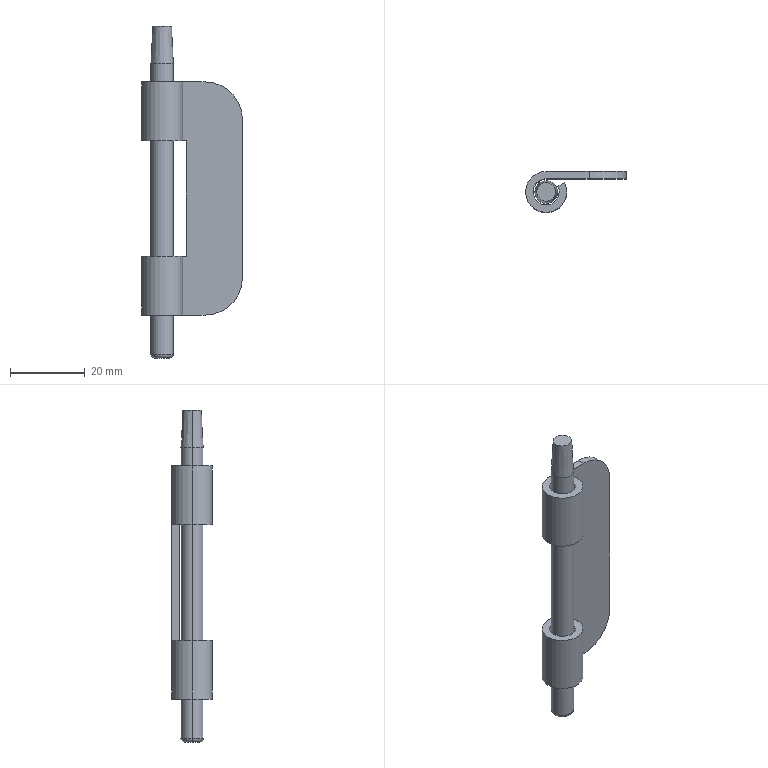Part | SolidWorks | features ICE 3, Chamfer 2, Fillet 2, ExtruThin 1 | 2 solids | 32 faces | box 27 x 11 x 89 mm | volume 6132 mm3 | cylinder 16 | plane 12 | torus 2 | cone 2 | commonest cylinder face diameters 7 x6 11 x6 6 x2 20 x2
STEP:
#1=CARTESIAN_POINT('',(-3.5,-3.5,31.25));
#2=VERTEX_POINT('',#1);
#3=CARTESIAN_POINT('',(3.5,-3.5,31.25));
#4=VERTEX_POINT('',#3);
#5=CARTESIAN_POINT('',(0.,-3.5,31.25));
#6=DIRECTION('',(0.,0.,1.));
#7=DIRECTION('',(1.,0.,0.));
#8=AXIS2_PLACEMENT_3D('',#5,#6,#7);
#9=CIRCLE('',#8,3.5);
#10=EDGE_CURVE('',#2,#4,#9,.T.);
#11=ORIENTED_EDGE('',*,*,#10,.T.);
#12=CARTESIAN_POINT('',(3.5,-3.5,15.5));
#13=VERTEX_POINT('',#12);
#14=CARTESIAN_POINT('',(3.5,-3.5,31.25));
#15=DIRECTION('',(0.,0.,-1.));
#16=VECTOR('',#15,1000.);
#17=LINE('',#14,#16);
#18=EDGE_CURVE('',#4,#13,#17,.T.);
#19=ORIENTED_EDGE('',*,*,#18,.T.);
#20=CARTESIAN_POINT('',(-3.5,-3.5,15.5));
#21=VERTEX_POINT('',#20);
#22=CARTESIAN_POINT('',(0.,-3.5,15.5));
#23=DIRECTION('',(0.,0.,1.));
#24=DIRECTION('',(1.,0.,0.));
#25=AXIS2_PLACEMENT_3D('',#22,#23,#24);
#26=CIRCLE('',#25,3.5);
#27=EDGE_CURVE('',#21,#13,#26,.T.);
#28=ORIENTED_EDGE('',*,*,#27,.F.);
#29=CARTESIAN_POINT('',(-3.5,-3.5,31.25));
#30=DIRECTION('',(0.,0.,-1.));
#31=VECTOR('',#30,1000.);
#32=LINE('',#29,#31);
#33=EDGE_CURVE('',#2,#21,#32,.T.);
#34=ORIENTED_EDGE('',*,*,#33,.F.);
#35=EDGE_LOOP('',(#11,#19,#28,#34));
#36=FACE_OUTER_BOUND('',#35,.T.);
#37=CARTESIAN_POINT('',(0.,-3.5,31.25));
#38=DIRECTION('',(0.,0.,-1.));
#39=DIRECTION('',(-1.,0.,0.));
#40=AXIS2_PLACEMENT_3D('',#37,#38,#39);
#41=CYLINDRICAL_SURFACE('',#40,3.5);
#42=ADVANCED_FACE('',(#36),#41,.F.);
#43=CARTESIAN_POINT('',(0.,0.,31.25));
#44=VERTEX_POINT('',#43);
#45=CARTESIAN_POINT('',(0.,-3.5,31.25));
#46=DIRECTION('',(0.,0.,1.));
#47=DIRECTION('',(1.,0.,0.));
#48=AXIS2_PLACEMENT_3D('',#45,#46,#47);
#49=CIRCLE('',#48,3.5);
#50=EDGE_CURVE('',#44,#2,#49,.T.);
#51=ORIENTED_EDGE('',*,*,#50,.T.);
#52=ORIENTED_EDGE('',*,*,#33,.T.);
#53=CARTESIAN_POINT('',(0.,0.,15.5));
#54=VERTEX_POINT('',#53);
#55=CARTESIAN_POINT('',(0.,-3.5,15.5));
#56=DIRECTION('',(0.,0.,1.));
#57=DIRECTION('',(1.,0.,0.));
#58=AXIS2_PLACEMENT_3D('',#55,#56,#57);
#59=CIRCLE('',#58,3.5);
#60=EDGE_CURVE('',#54,#21,#59,.T.);
#61=ORIENTED_EDGE('',*,*,#60,.F.);
#62=CARTESIAN_POINT('',(0.,0.,31.25));
#63=DIRECTION('',(0.,0.,-1.));
#64=VECTOR('',#63,1000.);
#65=LINE('',#62,#64);
#66=EDGE_CURVE('',#44,#54,#65,.T.);
#67=ORIENTED_EDGE('',*,*,#66,.F.);
#68=EDGE_LOOP('',(#51,#52,#61,#67));
#69=FACE_OUTER_BOUND('',#68,.T.);
#70=CARTESIAN_POINT('',(0.,-3.5,31.25));
#71=DIRECTION('',(0.,0.,-1.));
#72=DIRECTION('',(-1.,0.,0.));
#73=AXIS2_PLACEMENT_3D('',#70,#71,#72);
#74=CYLINDRICAL_SURFACE('',#73,3.5);
#75=ADVANCED_FACE('',(#69),#74,.F.);
#76=CARTESIAN_POINT('',(4.939,-1.08,-15.5));
#77=VERTEX_POINT('',#76);
#78=CARTESIAN_POINT('',(5.5,-3.5,-15.5));
#79=VERTEX_POINT('',#78);
#80=CARTESIAN_POINT('',(0.,-3.5,-15.5));
#81=DIRECTION('',(0.,0.,-1.));
#82=DIRECTION('',(-1.,0.,0.));
#83=AXIS2_PLACEMENT_3D('',#80,#81,#82);
#84=CIRCLE('',#83,5.5);
#85=EDGE_CURVE('',#77,#79,#84,.T.);
#86=ORIENTED_EDGE('',*,*,#85,.T.);
#87=CARTESIAN_POINT('',(5.5,-3.5,-31.25));
#88=VERTEX_POINT('',#87);
#89=CARTESIAN_POINT('',(5.5,-3.5,31.25));
#90=DIRECTION('',(0.,0.,-1.));
#91=VECTOR('',#90,1000.);
#92=LINE('',#89,#91);
#93=EDGE_CURVE('',#79,#88,#92,.T.);
#94=ORIENTED_EDGE('',*,*,#93,.T.);
#95=CARTESIAN_POINT('',(4.939,-1.08,-31.25));
#96=VERTEX_POINT('',#95);
#97=CARTESIAN_POINT('',(0.,-3.5,-31.25));
#98=DIRECTION('',(0.,0.,1.));
#99=DIRECTION('',(1.,0.,0.));
#100=AXIS2_PLACEMENT_3D('',#97,#98,#99);
#101=CIRCLE('',#100,5.5);
#102=EDGE_CURVE('',#88,#96,#101,.T.);
#103=ORIENTED_EDGE('',*,*,#102,.T.);
#104=CARTESIAN_POINT('',(4.939,-1.08,31.25));
#105=DIRECTION('',(0.,0.,-1.));
#106=VECTOR('',#105,1000.);
#107=LINE('',#104,#106);
#108=EDGE_CURVE('',#77,#96,#107,.T.);
#109=ORIENTED_EDGE('',*,*,#108,.F.);
#110=EDGE_LOOP('',(#86,#94,#103,#109));
#111=FACE_OUTER_BOUND('',#110,.T.);
#112=CARTESIAN_POINT('',(0.,-3.5,31.25));
#113=DIRECTION('',(0.,0.,-1.));
#114=DIRECTION('',(-1.,0.,0.));
#115=AXIS2_PLACEMENT_3D('',#112,#113,#114);
#116=CYLINDRICAL_SURFACE('',#115,5.5);
#117=ADVANCED_FACE('',(#111),#116,.T.);
#118=ORIENTED_EDGE('',*,*,#93,.F.);
#119=CARTESIAN_POINT('',(-5.5,-3.5,-15.5));
#120=VERTEX_POINT('',#119);
#121=CARTESIAN_POINT('',(0.,-3.5,-15.5));
#122=DIRECTION('',(0.,0.,-1.));
#123=DIRECTION('',(-1.,0.,0.));
#124=AXIS2_PLACEMENT_3D('',#121,#122,#123);
#125=CIRCLE('',#124,5.5);
#126=EDGE_CURVE('',#79,#120,#125,.T.);
#127=ORIENTED_EDGE('',*,*,#126,.T.);
#128=CARTESIAN_POINT('',(-5.5,-3.5,-31.25));
#129=VERTEX_POINT('',#128);
#130=CARTESIAN_POINT('',(-5.5,-3.5,31.25));
#131=DIRECTION('',(0.,0.,-1.));
#132=VECTOR('',#131,1000.);
#133=LINE('',#130,#132);
#134=EDGE_CURVE('',#120,#129,#133,.T.);
#135=ORIENTED_EDGE('',*,*,#134,.T.);
#136=CARTESIAN_POINT('',(0.,-3.5,-31.25));
#137=DIRECTION('',(0.,0.,1.));
#138=DIRECTION('',(1.,0.,0.));
#139=AXIS2_PLACEMENT_3D('',#136,#137,#138);
#140=CIRCLE('',#139,5.5);
#141=EDGE_CURVE('',#129,#88,#140,.T.);
#142=ORIENTED_EDGE('',*,*,#141,.T.);
#143=EDGE_LOOP('',(#118,#127,#135,#142));
#144=FACE_OUTER_BOUND('',#143,.T.);
#145=CARTESIAN_POINT('',(0.,-3.5,31.25));
#146=DIRECTION('',(0.,0.,-1.));
#147=DIRECTION('',(-1.,0.,0.));
#148=AXIS2_PLACEMENT_3D('',#145,#146,#147);
#149=CYLINDRICAL_SURFACE('',#148,5.5);
#150=ADVANCED_FACE('',(#144),#149,.T.);
#151=CARTESIAN_POINT('',(3.5,-3.5,-15.5));
#152=VERTEX_POINT('',#151);
#153=CARTESIAN_POINT('',(-3.5,-3.5,-15.5));
#154=VERTEX_POINT('',#153);
#155=CARTESIAN_POINT('',(0.,-3.5,-15.5));
#156=DIRECTION('',(0.,0.,-1.));
#157=DIRECTION('',(-1.,0.,0.));
#158=AXIS2_PLACEMENT_3D('',#155,#156,#157);
#159=CIRCLE('',#158,3.5);
#160=EDGE_CURVE('',#152,#154,#159,.T.);
#161=ORIENTED_EDGE('',*,*,#160,.F.);
#162=CARTESIAN_POINT('',(3.5,-3.5,-31.25));
#163=VERTEX_POINT('',#162);
#164=CARTESIAN_POINT('',(3.5,-3.5,31.25));
#165=DIRECTION('',(0.,0.,-1.));
#166=VECTOR('',#165,1000.);
#167=LINE('',#164,#166);
#168=EDGE_CURVE('',#152,#163,#167,.T.);
#169=ORIENTED_EDGE('',*,*,#168,.T.);
#170=CARTESIAN_POINT('',(-3.5,-3.5,-31.25));
#171=VERTEX_POINT('',#170);
#172=CARTESIAN_POINT('',(0.,-3.5,-31.25));
#173=DIRECTION('',(0.,0.,1.));
#174=DIRECTION('',(1.,0.,0.));
#175=AXIS2_PLACEMENT_3D('',#172,#173,#174);
#176=CIRCLE('',#175,3.5);
#177=EDGE_CURVE('',#171,#163,#176,.T.);
#178=ORIENTED_EDGE('',*,*,#177,.F.);
#179=CARTESIAN_POINT('',(-3.5,-3.5,31.25));
#180=DIRECTION('',(0.,0.,-1.));
#181=VECTOR('',#180,1000.);
#182=LINE('',#179,#181);
#183=EDGE_CURVE('',#154,#171,#182,.T.);
#184=ORIENTED_EDGE('',*,*,#183,.F.);
#185=EDGE_LOOP('',(#161,#169,#178,#184));
#186=FACE_OUTER_BOUND('',#185,.T.);
#187=CARTESIAN_POINT('',(0.,-3.5,31.25));
#188=DIRECTION('',(0.,0.,-1.));
#189=DIRECTION('',(-1.,0.,0.));
#190=AXIS2_PLACEMENT_3D('',#187,#188,#189);
#191=CYLINDRICAL_SURFACE('',#190,3.5);
#192=ADVANCED_FACE('',(#186),#191,.F.);
#193=CARTESIAN_POINT('',(0.,0.,-15.5));
#194=VERTEX_POINT('',#193);
#195=CARTESIAN_POINT('',(0.,-3.5,-15.5));
#196=DIRECTION('',(0.,0.,-1.));
#197=DIRECTION('',(-1.,0.,0.));
#198=AXIS2_PLACEMENT_3D('',#195,#196,#197);
#199=CIRCLE('',#198,3.5);
#200=EDGE_CURVE('',#154,#194,#199,.T.);
#201=ORIENTED_EDGE('',*,*,#200,.F.);
#202=ORIENTED_EDGE('',*,*,#183,.T.);
#203=CARTESIAN_POINT('',(0.,0.,-31.25));
#204=VERTEX_POINT('',#203);
#205=CARTESIAN_POINT('',(0.,-3.5,-31.25));
#206=DIRECTION('',(0.,0.,1.));
#207=DIRECTION('',(1.,0.,0.));
#208=AXIS2_PLACEMENT_3D('',#205,#206,#207);
#209=CIRCLE('',#208,3.5);
#210=EDGE_CURVE('',#204,#171,#209,.T.);
#211=ORIENTED_EDGE('',*,*,#210,.F.);
#212=CARTESIAN_POINT('',(0.,0.,31.25));
#213=DIRECTION('',(0.,0.,-1.));
#214=VECTOR('',#213,1000.);
#215=LINE('',#212,#214);
#216=EDGE_CURVE('',#194,#204,#215,.T.);
#217=ORIENTED_EDGE('',*,*,#216,.F.);
#218=EDGE_LOOP('',(#201,#202,#211,#217));
#219=FACE_OUTER_BOUND('',#218,.T.);
#220=CARTESIAN_POINT('',(0.,-3.5,31.25));
#221=DIRECTION('',(0.,0.,-1.));
#222=DIRECTION('',(-1.,0.,0.));
#223=AXIS2_PLACEMENT_3D('',#220,#221,#222);
#224=CYLINDRICAL_SURFACE('',#223,3.5);
#225=ADVANCED_FACE('',(#219),#224,.F.);
#226=CARTESIAN_POINT('',(5.5,-3.5,31.25));
#227=VERTEX_POINT('',#226);
#228=CARTESIAN_POINT('',(4.939,-1.08,31.25));
#229=VERTEX_POINT('',#228);
#230=CARTESIAN_POINT('',(0.,-3.5,31.25));
#231=DIRECTION('',(0.,0.,1.));
#232=DIRECTION('',(1.,0.,0.));
#233=AXIS2_PLACEMENT_3D('',#230,#231,#232);
#234=CIRCLE('',#233,5.5);
#235=EDGE_CURVE('',#227,#229,#234,.T.);
#236=ORIENTED_EDGE('',*,*,#235,.F.);
#237=CARTESIAN_POINT('',(5.5,-3.5,15.5));
#238=VERTEX_POINT('',#237);
#239=CARTESIAN_POINT('',(5.5,-3.5,31.25));
#240=DIRECTION('',(0.,0.,-1.));
#241=VECTOR('',#240,1000.);
#242=LINE('',#239,#241);
#243=EDGE_CURVE('',#227,#238,#242,.T.);
#244=ORIENTED_EDGE('',*,*,#243,.T.);
#245=CARTESIAN_POINT('',(4.939,-1.08,15.5));
#246=VERTEX_POINT('',#245);
#247=CARTESIAN_POINT('',(0.,-3.5,15.5));
#248=DIRECTION('',(0.,0.,1.));
#249=DIRECTION('',(1.,0.,0.));
#250=AXIS2_PLACEMENT_3D('',#247,#248,#249);
#251=CIRCLE('',#250,5.5);
#252=EDGE_CURVE('',#238,#246,#251,.T.);
#253=ORIENTED_EDGE('',*,*,#252,.T.);
#254=CARTESIAN_POINT('',(4.939,-1.08,31.25));
#255=DIRECTION('',(0.,0.,-1.));
#256=VECTOR('',#255,1000.);
#257=LINE('',#254,#256);
#258=EDGE_CURVE('',#229,#246,#257,.T.);
#259=ORIENTED_EDGE('',*,*,#258,.F.);
#260=EDGE_LOOP('',(#236,#244,#253,#259));
#261=FACE_OUTER_BOUND('',#260,.T.);
#262=CARTESIAN_POINT('',(0.,-3.5,31.25));
#263=DIRECTION('',(0.,0.,-1.));
#264=DIRECTION('',(-1.,0.,0.));
#265=AXIS2_PLACEMENT_3D('',#262,#263,#264);
#266=CYLINDRICAL_SURFACE('',#265,5.5);
#267=ADVANCED_FACE('',(#261),#266,.T.);
#268=ORIENTED_EDGE('',*,*,#243,.F.);
#269=CARTESIAN_POINT('',(-5.5,-3.5,31.25));
#270=VERTEX_POINT('',#269);
#271=CARTESIAN_POINT('',(0.,-3.5,31.25));
#272=DIRECTION('',(0.,0.,1.));
#273=DIRECTION('',(1.,0.,0.));
#274=AXIS2_PLACEMENT_3D('',#271,#272,#273);
#275=CIRCLE('',#274,5.5);
#276=EDGE_CURVE('',#270,#227,#275,.T.);
#277=ORIENTED_EDGE('',*,*,#276,.F.);
#278=CARTESIAN_POINT('',(-5.5,-3.5,15.5));
#279=VERTEX_POINT('',#278);
#280=CARTESIAN_POINT('',(-5.5,-3.5,31.25));
#281=DIRECTION('',(0.,0.,-1.));
#282=VECTOR('',#281,1000.);
#283=LINE('',#280,#282);
#284=EDGE_CURVE('',#270,#279,#283,.T.);
#285=ORIENTED_EDGE('',*,*,#284,.T.);
#286=CARTESIAN_POINT('',(0.,-3.5,15.5));
#287=DIRECTION('',(0.,0.,1.));
#288=DIRECTION('',(1.,0.,0.));
#289=AXIS2_PLACEMENT_3D('',#286,#287,#288);
#290=CIRCLE('',#289,5.5);
#291=EDGE_CURVE('',#279,#238,#290,.T.);
#292=ORIENTED_EDGE('',*,*,#291,.T.);
#293=EDGE_LOOP('',(#268,#277,#285,#292));
#294=FACE_OUTER_BOUND('',#293,.T.);
#295=CARTESIAN_POINT('',(0.,-3.5,31.25));
#296=DIRECTION('',(0.,0.,-1.));
#297=DIRECTION('',(-1.,0.,0.));
#298=AXIS2_PLACEMENT_3D('',#295,#296,#297);
#299=CYLINDRICAL_SURFACE('',#298,5.5);
#300=ADVANCED_FACE('',(#294),#299,.T.);
#301=ORIENTED_EDGE('',*,*,#284,.F.);
#302=CARTESIAN_POINT('',(0.,2.,31.25));
#303=VERTEX_POINT('',#302);
#304=CARTESIAN_POINT('',(0.,-3.5,31.25));
#305=DIRECTION('',(0.,0.,1.));
#306=DIRECTION('',(1.,0.,0.));
#307=AXIS2_PLACEMENT_3D('',#304,#305,#306);
#308=CIRCLE('',#307,5.5);
#309=EDGE_CURVE('',#303,#270,#308,.T.);
#310=ORIENTED_EDGE('',*,*,#309,.F.);
#311=CARTESIAN_POINT('',(0.,2.,15.5));
#312=VERTEX_POINT('',#311);
#313=CARTESIAN_POINT('',(0.,2.,31.25));
#314=DIRECTION('',(0.,0.,-1.));
#315=VECTOR('',#314,1000.);
#316=LINE('',#313,#315);
#317=EDGE_CURVE('',#303,#312,#316,.T.);
#318=ORIENTED_EDGE('',*,*,#317,.T.);
#319=CARTESIAN_POINT('',(0.,-3.5,15.5));
#320=DIRECTION('',(0.,0.,1.));
#321=DIRECTION('',(1.,0.,0.));
#322=AXIS2_PLACEMENT_3D('',#319,#320,#321);
#323=CIRCLE('',#322,5.5);
#324=EDGE_CURVE('',#312,#279,#323,.T.);
#325=ORIENTED_EDGE('',*,*,#324,.T.);
#326=EDGE_LOOP('',(#301,#310,#318,#325));
#327=FACE_OUTER_BOUND('',#326,.T.);
#328=CARTESIAN_POINT('',(0.,-3.5,31.25));
#329=DIRECTION('',(0.,0.,-1.));
#330=DIRECTION('',(-1.,0.,0.));
#331=AXIS2_PLACEMENT_3D('',#328,#329,#330);
#332=CYLINDRICAL_SURFACE('',#331,5.5);
#333=ADVANCED_FACE('',(#327),#332,.T.);
#334=CARTESIAN_POINT('',(3.143,-1.96,-15.5));
#335=VERTEX_POINT('',#334);
#336=CARTESIAN_POINT('',(3.143,-1.96,-15.5));
#337=DIRECTION('',(-0.898,-0.44,0.));
#338=VECTOR('',#337,1000.);
#339=LINE('',#336,#338);
#340=EDGE_CURVE('',#77,#335,#339,.T.);
#341=ORIENTED_EDGE('',*,*,#340,.F.);
#342=ORIENTED_EDGE('',*,*,#108,.T.);
#343=CARTESIAN_POINT('',(3.143,-1.96,-31.25));
#344=VERTEX_POINT('',#343);
#345=CARTESIAN_POINT('',(3.143,-1.96,-31.25));
#346=DIRECTION('',(0.898,0.44,0.));
#347=VECTOR('',#346,1000.);
#348=LINE('',#345,#347);
#349=EDGE_CURVE('',#344,#96,#348,.T.);
#350=ORIENTED_EDGE('',*,*,#349,.F.);
#351=CARTESIAN_POINT('',(3.143,-1.96,31.25));
#352=DIRECTION('',(0.,0.,-1.));
#353=VECTOR('',#352,1000.);
#354=LINE('',#351,#353);
#355=EDGE_CURVE('',#335,#344,#354,.T.);
#356=ORIENTED_EDGE('',*,*,#355,.F.);
#357=EDGE_LOOP('',(#341,#342,#350,#356));
#358=FACE_OUTER_BOUND('',#357,.T.);
#359=CARTESIAN_POINT('',(3.143,-1.96,31.25));
#360=DIRECTION('',(-0.44,0.898,0.));
#361=DIRECTION('',(-0.898,-0.44,0.));
#362=AXIS2_PLACEMENT_3D('',#359,#360,#361);
#363=PLANE('',#362);
#364=ADVANCED_FACE('',(#358),#363,.T.);
#365=ORIENTED_EDGE('',*,*,#168,.F.);
#366=CARTESIAN_POINT('',(0.,-3.5,-15.5));
#367=DIRECTION('',(0.,0.,-1.));
#368=DIRECTION('',(-1.,0.,0.));
#369=AXIS2_PLACEMENT_3D('',#366,#367,#368);
#370=CIRCLE('',#369,3.5);
#371=EDGE_CURVE('',#335,#152,#370,.T.);
#372=ORIENTED_EDGE('',*,*,#371,.F.);
#373=ORIENTED_EDGE('',*,*,#355,.T.);
#374=CARTESIAN_POINT('',(0.,-3.5,-31.25));
#375=DIRECTION('',(0.,0.,1.));
#376=DIRECTION('',(1.,0.,0.));
#377=AXIS2_PLACEMENT_3D('',#374,#375,#376);
#378=CIRCLE('',#377,3.5);
#379=EDGE_CURVE('',#163,#344,#378,.T.);
#380=ORIENTED_EDGE('',*,*,#379,.F.);
#381=EDGE_LOOP('',(#365,#372,#373,#380));
#382=FACE_OUTER_BOUND('',#381,.T.);
#383=CARTESIAN_POINT('',(0.,-3.5,31.25));
#384=DIRECTION('',(0.,0.,-1.));
#385=DIRECTION('',(-1.,0.,0.));
#386=AXIS2_PLACEMENT_3D('',#383,#384,#385);
#387=CYLINDRICAL_SURFACE('',#386,3.5);
#388=ADVANCED_FACE('',(#382),#387,.F.);
#389=ORIENTED_EDGE('',*,*,#134,.F.);
#390=CARTESIAN_POINT('',(0.,2.,-15.5));
#391=VERTEX_POINT('',#390);
#392=CARTESIAN_POINT('',(0.,-3.5,-15.5));
#393=DIRECTION('',(0.,0.,-1.));
#394=DIRECTION('',(-1.,0.,0.));
#395=AXIS2_PLACEMENT_3D('',#392,#393,#394);
#396=CIRCLE('',#395,5.5);
#397=EDGE_CURVE('',#120,#391,#396,.T.);
#398=ORIENTED_EDGE('',*,*,#397,.T.);
#399=CARTESIAN_POINT('',(0.,2.,-31.25));
#400=VERTEX_POINT('',#399);
#401=CARTESIAN_POINT('',(0.,2.,31.25));
#402=DIRECTION('',(0.,0.,-1.));
#403=VECTOR('',#402,1000.);
#404=LINE('',#401,#403);
#405=EDGE_CURVE('',#391,#400,#404,.T.);
#406=ORIENTED_EDGE('',*,*,#405,.T.);
#407=CARTESIAN_POINT('',(0.,-3.5,-31.25));
#408=DIRECTION('',(0.,0.,1.));
#409=DIRECTION('',(1.,0.,0.));
#410=AXIS2_PLACEMENT_3D('',#407,#408,#409);
#411=CIRCLE('',#410,5.5);
#412=EDGE_CURVE('',#400,#129,#411,.T.);
#413=ORIENTED_EDGE('',*,*,#412,.T.);
#414=EDGE_LOOP('',(#389,#398,#406,#413));
#415=FACE_OUTER_BOUND('',#414,.T.);
#416=CARTESIAN_POINT('',(0.,-3.5,31.25));
#417=DIRECTION('',(0.,0.,-1.));
#418=DIRECTION('',(-1.,0.,0.));
#419=AXIS2_PLACEMENT_3D('',#416,#417,#418);
#420=CYLINDRICAL_SURFACE('',#419,5.5);
#421=ADVANCED_FACE('',(#415),#420,.T.);
#422=CARTESIAN_POINT('',(3.143,-1.96,15.5));
#423=VERTEX_POINT('',#422);
#424=CARTESIAN_POINT('',(3.143,-1.96,15.5));
#425=DIRECTION('',(0.898,0.44,0.));
#426=VECTOR('',#425,1000.);
#427=LINE('',#424,#426);
#428=EDGE_CURVE('',#423,#246,#427,.T.);
#429=ORIENTED_EDGE('',*,*,#428,.F.);
#430=CARTESIAN_POINT('',(3.143,-1.96,31.25));
#431=VERTEX_POINT('',#430);
#432=CARTESIAN_POINT('',(3.143,-1.96,31.25));
#433=DIRECTION('',(0.,0.,-1.));
#434=VECTOR('',#433,1000.);
#435=LINE('',#432,#434);
#436=EDGE_CURVE('',#431,#423,#435,.T.);
#437=ORIENTED_EDGE('',*,*,#436,.F.);
#438=CARTESIAN_POINT('',(3.143,-1.96,31.25));
#439=DIRECTION('',(0.898,0.44,0.));
#440=VECTOR('',#439,1000.);
#441=LINE('',#438,#440);
#442=EDGE_CURVE('',#431,#229,#441,.T.);
#443=ORIENTED_EDGE('',*,*,#442,.T.);
#444=ORIENTED_EDGE('',*,*,#258,.T.);
#445=EDGE_LOOP('',(#429,#437,#443,#444));
#446=FACE_OUTER_BOUND('',#445,.T.);
#447=CARTESIAN_POINT('',(3.143,-1.96,31.25));
#448=DIRECTION('',(-0.44,0.898,0.));
#449=DIRECTION('',(-0.898,-0.44,0.));
#450=AXIS2_PLACEMENT_3D('',#447,#448,#449);
#451=PLANE('',#450);
#452=ADVANCED_FACE('',(#446),#451,.T.);
#453=ORIENTED_EDGE('',*,*,#18,.F.);
#454=CARTESIAN_POINT('',(0.,-3.5,31.25));
#455=DIRECTION('',(0.,0.,1.));
#456=DIRECTION('',(1.,0.,0.));
#457=AXIS2_PLACEMENT_3D('',#454,#455,#456);
#458=CIRCLE('',#457,3.5);
#459=EDGE_CURVE('',#4,#431,#458,.T.);
#460=ORIENTED_EDGE('',*,*,#459,.T.);
#461=ORIENTED_EDGE('',*,*,#436,.T.);
#462=CARTESIAN_POINT('',(0.,-3.5,15.5));
#463=DIRECTION('',(0.,0.,1.));
#464=DIRECTION('',(1.,0.,0.));
#465=AXIS2_PLACEMENT_3D('',#462,#463,#464);
#466=CIRCLE('',#465,3.5);
#467=EDGE_CURVE('',#13,#423,#466,.T.);
#468=ORIENTED_EDGE('',*,*,#467,.F.);
#469=EDGE_LOOP('',(#453,#460,#461,#468));
#470=FACE_OUTER_BOUND('',#469,.T.);
#471=CARTESIAN_POINT('',(0.,-3.5,31.25));
#472=DIRECTION('',(0.,0.,-1.));
#473=DIRECTION('',(-1.,0.,0.));
#474=AXIS2_PLACEMENT_3D('',#471,#472,#473);
#475=CYLINDRICAL_SURFACE('',#474,3.5);
#476=ADVANCED_FACE('',(#470),#475,.F.);
#477=CARTESIAN_POINT('',(11.5,0.,-31.25));
#478=VERTEX_POINT('',#477);
#479=CARTESIAN_POINT('',(21.5,0.,-31.25));
#480=DIRECTION('',(-1.,0.,0.));
#481=VECTOR('',#480,1000.);
#482=LINE('',#479,#481);
#483=EDGE_CURVE('',#478,#204,#482,.T.);
#484=ORIENTED_EDGE('',*,*,#483,.F.);
#485=CARTESIAN_POINT('',(21.5,0.,-21.25));
#486=VERTEX_POINT('',#485);
#487=CARTESIAN_POINT('',(11.5,0.,-21.25));
#488=DIRECTION('',(0.,-1.,0.));
#489=DIRECTION('',(1.,0.,0.));
#490=AXIS2_PLACEMENT_3D('',#487,#488,#489);
#491=CIRCLE('',#490,10.);
#492=EDGE_CURVE('',#478,#486,#491,.T.);
#493=ORIENTED_EDGE('',*,*,#492,.T.);
#494=CARTESIAN_POINT('',(21.5,0.,21.25));
#495=VERTEX_POINT('',#494);
#496=CARTESIAN_POINT('',(21.5,0.,31.25));
#497=DIRECTION('',(0.,0.,-1.));
#498=VECTOR('',#497,1000.);
#499=LINE('',#496,#498);
#500=EDGE_CURVE('',#495,#486,#499,.T.);
#501=ORIENTED_EDGE('',*,*,#500,.F.);
#502=CARTESIAN_POINT('',(11.5,0.,31.25));
#503=VERTEX_POINT('',#502);
#504=CARTESIAN_POINT('',(11.5,0.,21.25));
#505=DIRECTION('',(0.,-1.,0.));
#506=DIRECTION('',(1.,0.,0.));
#507=AXIS2_PLACEMENT_3D('',#504,#505,#506);
#508=CIRCLE('',#507,10.);
#509=EDGE_CURVE('',#495,#503,#508,.T.);
#510=ORIENTED_EDGE('',*,*,#509,.T.);
#511=CARTESIAN_POINT('',(21.5,0.,31.25));
#512=DIRECTION('',(-1.,0.,0.));
#513=VECTOR('',#512,1000.);
#514=LINE('',#511,#513);
#515=EDGE_CURVE('',#503,#44,#514,.T.);
#516=ORIENTED_EDGE('',*,*,#515,.T.);
#517=ORIENTED_EDGE('',*,*,#66,.T.);
#518=CARTESIAN_POINT('',(6.5,0.,15.5));
#519=VERTEX_POINT('',#518);
#520=CARTESIAN_POINT('',(21.5,0.,15.5));
#521=DIRECTION('',(-1.,0.,0.));
#522=VECTOR('',#521,1000.);
#523=LINE('',#520,#522);
#524=EDGE_CURVE('',#519,#54,#523,.T.);
#525=ORIENTED_EDGE('',*,*,#524,.F.);
#526=CARTESIAN_POINT('',(6.5,0.,-15.5));
#527=VERTEX_POINT('',#526);
#528=CARTESIAN_POINT('',(6.5,0.,31.25));
#529=DIRECTION('',(0.,0.,1.));
#530=VECTOR('',#529,1000.);
#531=LINE('',#528,#530);
#532=EDGE_CURVE('',#527,#519,#531,.T.);
#533=ORIENTED_EDGE('',*,*,#532,.F.);
#534=CARTESIAN_POINT('',(21.5,0.,-15.5));
#535=DIRECTION('',(1.,0.,0.));
#536=VECTOR('',#535,1000.);
#537=LINE('',#534,#536);
#538=EDGE_CURVE('',#194,#527,#537,.T.);
#539=ORIENTED_EDGE('',*,*,#538,.F.);
#540=ORIENTED_EDGE('',*,*,#216,.T.);
#541=EDGE_LOOP('',(#484,#493,#501,#510,#516,#517,#525,#533,#539,#540));
#542=FACE_OUTER_BOUND('',#541,.T.);
#543=CARTESIAN_POINT('',(21.5,0.,31.25));
#544=DIRECTION('',(0.,-1.,0.));
#545=DIRECTION('',(1.,0.,0.));
#546=AXIS2_PLACEMENT_3D('',#543,#544,#545);
#547=PLANE('',#546);
#548=ADVANCED_FACE('',(#542),#547,.T.);
#549=ORIENTED_EDGE('',*,*,#500,.T.);
#550=CARTESIAN_POINT('',(21.5,2.,-21.25));
#551=VERTEX_POINT('',#550);
#552=CARTESIAN_POINT('',(21.5,2.,-21.25));
#553=DIRECTION('',(0.,1.,0.));
#554=VECTOR('',#553,1000.);
#555=LINE('',#552,#554);
#556=EDGE_CURVE('',#486,#551,#555,.T.);
#557=ORIENTED_EDGE('',*,*,#556,.T.);
#558=CARTESIAN_POINT('',(21.5,2.,21.25));
#559=VERTEX_POINT('',#558);
#560=CARTESIAN_POINT('',(21.5,2.,31.25));
#561=DIRECTION('',(0.,0.,-1.));
#562=VECTOR('',#561,1000.);
#563=LINE('',#560,#562);
#564=EDGE_CURVE('',#559,#551,#563,.T.);
#565=ORIENTED_EDGE('',*,*,#564,.F.);
#566=CARTESIAN_POINT('',(21.5,2.,21.25));
#567=DIRECTION('',(0.,-1.,0.));
#568=VECTOR('',#567,1000.);
#569=LINE('',#566,#568);
#570=EDGE_CURVE('',#559,#495,#569,.T.);
#571=ORIENTED_EDGE('',*,*,#570,.T.);
#572=EDGE_LOOP('',(#549,#557,#565,#571));
#573=FACE_OUTER_BOUND('',#572,.T.);
#574=CARTESIAN_POINT('',(21.5,2.,31.25));
#575=DIRECTION('',(1.,0.,0.));
#576=DIRECTION('',(0.,0.,-1.));
#577=AXIS2_PLACEMENT_3D('',#574,#575,#576);
#578=PLANE('',#577);
#579=ADVANCED_FACE('',(#573),#578,.T.);
#580=ORIENTED_EDGE('',*,*,#564,.T.);
#581=CARTESIAN_POINT('',(11.5,2.,-31.25));
#582=VERTEX_POINT('',#581);
#583=CARTESIAN_POINT('',(11.5,2.,-21.25));
#584=DIRECTION('',(0.,1.,0.));
#585=DIRECTION('',(1.,0.,0.));
#586=AXIS2_PLACEMENT_3D('',#583,#584,#585);
#587=CIRCLE('',#586,10.);
#588=EDGE_CURVE('',#551,#582,#587,.T.);
#589=ORIENTED_EDGE('',*,*,#588,.T.);
#590=CARTESIAN_POINT('',(21.5,2.,-31.25));
#591=DIRECTION('',(-1.,0.,0.));
#592=VECTOR('',#591,1000.);
#593=LINE('',#590,#592);
#594=EDGE_CURVE('',#582,#400,#593,.T.);
#595=ORIENTED_EDGE('',*,*,#594,.T.);
#596=ORIENTED_EDGE('',*,*,#405,.F.);
#597=CARTESIAN_POINT('',(6.5,2.,-15.5));
#598=VERTEX_POINT('',#597);
#599=CARTESIAN_POINT('',(-5.5,2.,-15.5));
#600=DIRECTION('',(-1.,0.,0.));
#601=VECTOR('',#600,1000.);
#602=LINE('',#599,#601);
#603=EDGE_CURVE('',#598,#391,#602,.T.);
#604=ORIENTED_EDGE('',*,*,#603,.F.);
#605=CARTESIAN_POINT('',(6.5,2.,15.5));
#606=VERTEX_POINT('',#605);
#607=CARTESIAN_POINT('',(6.5,2.,-15.5));
#608=DIRECTION('',(0.,0.,-1.));
#609=VECTOR('',#608,1000.);
#610=LINE('',#607,#609);
#611=EDGE_CURVE('',#606,#598,#610,.T.);
#612=ORIENTED_EDGE('',*,*,#611,.F.);
#613=CARTESIAN_POINT('',(21.5,2.,15.5));
#614=DIRECTION('',(-1.,0.,0.));
#615=VECTOR('',#614,1000.);
#616=LINE('',#613,#615);
#617=EDGE_CURVE('',#606,#312,#616,.T.);
#618=ORIENTED_EDGE('',*,*,#617,.T.);
#619=ORIENTED_EDGE('',*,*,#317,.F.);
#620=CARTESIAN_POINT('',(11.5,2.,31.25));
#621=VERTEX_POINT('',#620);
#622=CARTESIAN_POINT('',(21.5,2.,31.25));
#623=DIRECTION('',(-1.,0.,0.));
#624=VECTOR('',#623,1000.);
#625=LINE('',#622,#624);
#626=EDGE_CURVE('',#621,#303,#625,.T.);
#627=ORIENTED_EDGE('',*,*,#626,.F.);
#628=CARTESIAN_POINT('',(11.5,2.,21.25));
#629=DIRECTION('',(0.,1.,0.));
#630=DIRECTION('',(1.,0.,0.));
#631=AXIS2_PLACEMENT_3D('',#628,#629,#630);
#632=CIRCLE('',#631,10.);
#633=EDGE_CURVE('',#621,#559,#632,.T.);
#634=ORIENTED_EDGE('',*,*,#633,.T.);
#635=EDGE_LOOP('',(#580,#589,#595,#596,#604,#612,#618,#619,#627,#634));
#636=FACE_OUTER_BOUND('',#635,.T.);
#637=CARTESIAN_POINT('',(21.5,2.,31.25));
#638=DIRECTION('',(0.,-1.,0.));
#639=DIRECTION('',(1.,0.,0.));
#640=AXIS2_PLACEMENT_3D('',#637,#638,#639);
#641=PLANE('',#640);
#642=ADVANCED_FACE('',(#636),#641,.F.);
#643=ORIENTED_EDGE('',*,*,#515,.F.);
#644=CARTESIAN_POINT('',(11.5,-3.5,31.25));
#645=DIRECTION('',(0.,1.,0.));
#646=VECTOR('',#645,1000.);
#647=LINE('',#644,#646);
#648=EDGE_CURVE('',#503,#621,#647,.T.);
#649=ORIENTED_EDGE('',*,*,#648,.T.);
#650=ORIENTED_EDGE('',*,*,#626,.T.);
#651=ORIENTED_EDGE('',*,*,#309,.T.);
#652=ORIENTED_EDGE('',*,*,#276,.T.);
#653=ORIENTED_EDGE('',*,*,#235,.T.);
#654=ORIENTED_EDGE('',*,*,#442,.F.);
#655=ORIENTED_EDGE('',*,*,#459,.F.);
#656=ORIENTED_EDGE('',*,*,#10,.F.);
#657=ORIENTED_EDGE('',*,*,#50,.F.);
#658=EDGE_LOOP('',(#643,#649,#650,#651,#652,#653,#654,#655,#656,#657));
#659=FACE_OUTER_BOUND('',#658,.T.);
#660=CARTESIAN_POINT('',(0.,-3.5,31.25));
#661=DIRECTION('',(0.,0.,1.));
#662=DIRECTION('',(1.,0.,0.));
#663=AXIS2_PLACEMENT_3D('',#660,#661,#662);
#664=PLANE('',#663);
#665=ADVANCED_FACE('',(#659),#664,.T.);
#666=ORIENTED_EDGE('',*,*,#594,.F.);
#667=CARTESIAN_POINT('',(11.5,0.,-31.25));
#668=DIRECTION('',(0.,-1.,0.));
#669=VECTOR('',#668,1000.);
#670=LINE('',#667,#669);
#671=EDGE_CURVE('',#582,#478,#670,.T.);
#672=ORIENTED_EDGE('',*,*,#671,.T.);
#673=ORIENTED_EDGE('',*,*,#483,.T.);
#674=ORIENTED_EDGE('',*,*,#210,.T.);
#675=ORIENTED_EDGE('',*,*,#177,.T.);
#676=ORIENTED_EDGE('',*,*,#379,.T.);
#677=ORIENTED_EDGE('',*,*,#349,.T.);
#678=ORIENTED_EDGE('',*,*,#102,.F.);
#679=ORIENTED_EDGE('',*,*,#141,.F.);
#680=ORIENTED_EDGE('',*,*,#412,.F.);
#681=EDGE_LOOP('',(#666,#672,#673,#674,#675,#676,#677,#678,#679,#680));
#682=FACE_OUTER_BOUND('',#681,.T.);
#683=CARTESIAN_POINT('',(0.,-3.5,-31.25));
#684=DIRECTION('',(0.,0.,1.));
#685=DIRECTION('',(1.,0.,0.));
#686=AXIS2_PLACEMENT_3D('',#683,#684,#685);
#687=PLANE('',#686);
#688=ADVANCED_FACE('',(#682),#687,.F.);
#689=ORIENTED_EDGE('',*,*,#85,.F.);
#690=ORIENTED_EDGE('',*,*,#340,.T.);
#691=ORIENTED_EDGE('',*,*,#371,.T.);
#692=ORIENTED_EDGE('',*,*,#160,.T.);
#693=ORIENTED_EDGE('',*,*,#200,.T.);
#694=ORIENTED_EDGE('',*,*,#538,.T.);
#695=CARTESIAN_POINT('',(6.5,-9.,-15.5));
#696=DIRECTION('',(0.,1.,0.));
#697=VECTOR('',#696,1000.);
#698=LINE('',#695,#697);
#699=EDGE_CURVE('',#527,#598,#698,.T.);
#700=ORIENTED_EDGE('',*,*,#699,.T.);
#701=ORIENTED_EDGE('',*,*,#603,.T.);
#702=ORIENTED_EDGE('',*,*,#397,.F.);
#703=ORIENTED_EDGE('',*,*,#126,.F.);
#704=EDGE_LOOP('',(#689,#690,#691,#692,#693,#694,#700,#701,#702,#703));
#705=FACE_OUTER_BOUND('',#704,.T.);
#706=CARTESIAN_POINT('',(-5.5,-9.,-15.5));
#707=DIRECTION('',(0.,0.,-1.));
#708=DIRECTION('',(-1.,0.,0.));
#709=AXIS2_PLACEMENT_3D('',#706,#707,#708);
#710=PLANE('',#709);
#711=ADVANCED_FACE('',(#705),#710,.F.);
#712=ORIENTED_EDGE('',*,*,#617,.F.);
#713=CARTESIAN_POINT('',(6.5,-9.,15.5));
#714=DIRECTION('',(0.,1.,0.));
#715=VECTOR('',#714,1000.);
#716=LINE('',#713,#715);
#717=EDGE_CURVE('',#519,#606,#716,.T.);
#718=ORIENTED_EDGE('',*,*,#717,.F.);
#719=ORIENTED_EDGE('',*,*,#524,.T.);
#720=ORIENTED_EDGE('',*,*,#60,.T.);
#721=ORIENTED_EDGE('',*,*,#27,.T.);
#722=ORIENTED_EDGE('',*,*,#467,.T.);
#723=ORIENTED_EDGE('',*,*,#428,.T.);
#724=ORIENTED_EDGE('',*,*,#252,.F.);
#725=ORIENTED_EDGE('',*,*,#291,.F.);
#726=ORIENTED_EDGE('',*,*,#324,.F.);
#727=EDGE_LOOP('',(#712,#718,#719,#720,#721,#722,#723,#724,#725,#726));
#728=FACE_OUTER_BOUND('',#727,.T.);
#729=CARTESIAN_POINT('',(-5.5,-9.,15.5));
#730=DIRECTION('',(0.,0.,1.));
#731=DIRECTION('',(1.,0.,0.));
#732=AXIS2_PLACEMENT_3D('',#729,#730,#731);
#733=PLANE('',#732);
#734=ADVANCED_FACE('',(#728),#733,.F.);
#735=ORIENTED_EDGE('',*,*,#532,.T.);
#736=ORIENTED_EDGE('',*,*,#717,.T.);
#737=ORIENTED_EDGE('',*,*,#611,.T.);
#738=ORIENTED_EDGE('',*,*,#699,.F.);
#739=EDGE_LOOP('',(#735,#736,#737,#738));
#740=FACE_OUTER_BOUND('',#739,.T.);
#741=CARTESIAN_POINT('',(6.5,-9.,-15.5));
#742=DIRECTION('',(1.,0.,0.));
#743=DIRECTION('',(0.,0.,-1.));
#744=AXIS2_PLACEMENT_3D('',#741,#742,#743);
#745=PLANE('',#744);
#746=ADVANCED_FACE('',(#740),#745,.F.);
#747=ORIENTED_EDGE('',*,*,#588,.F.);
#748=ORIENTED_EDGE('',*,*,#556,.F.);
#749=ORIENTED_EDGE('',*,*,#492,.F.);
#750=ORIENTED_EDGE('',*,*,#671,.F.);
#751=EDGE_LOOP('',(#747,#748,#749,#750));
#752=FACE_OUTER_BOUND('',#751,.T.);
#753=CARTESIAN_POINT('',(11.5,-3.5,-21.25));
#754=DIRECTION('',(0.,1.,0.));
#755=DIRECTION('',(0.,0.,1.));
#756=AXIS2_PLACEMENT_3D('',#753,#754,#755);
#757=CYLINDRICAL_SURFACE('',#756,10.);
#758=ADVANCED_FACE('',(#752),#757,.T.);
#759=ORIENTED_EDGE('',*,*,#633,.F.);
#760=ORIENTED_EDGE('',*,*,#648,.F.);
#761=ORIENTED_EDGE('',*,*,#509,.F.);
#762=ORIENTED_EDGE('',*,*,#570,.F.);
#763=EDGE_LOOP('',(#759,#760,#761,#762));
#764=FACE_OUTER_BOUND('',#763,.T.);
#765=CARTESIAN_POINT('',(11.5,2.,21.25));
#766=DIRECTION('',(0.,-1.,0.));
#767=DIRECTION('',(0.,0.,-1.));
#768=AXIS2_PLACEMENT_3D('',#765,#766,#767);
#769=CYLINDRICAL_SURFACE('',#768,10.);
#770=ADVANCED_FACE('',(#764),#769,.T.);
#771=CLOSED_SHELL('',(#42,#75,#117,#150,#192,#225,#267,#300,#333,#364,#388,#421,#452,#476,#548,#579,#642,#665,#688,#711,#734,#746,#758,#770));
#772=MANIFOLD_SOLID_BREP('',#771);
#773=CARTESIAN_POINT('',(3.,-3.5,-41.75));
#774=VERTEX_POINT('',#773);
#775=CARTESIAN_POINT('',(-3.,-3.5,-41.75));
#776=VERTEX_POINT('',#775);
#777=CARTESIAN_POINT('',(0.,-3.5,-41.75));
#778=DIRECTION('',(0.,0.,1.));
#779=DIRECTION('',(-1.,0.,0.));
#780=AXIS2_PLACEMENT_3D('',#777,#778,#779);
#781=CIRCLE('',#780,3.);
#782=EDGE_CURVE('',#774,#776,#781,.T.);
#783=ORIENTED_EDGE('',*,*,#782,.F.);
#784=CARTESIAN_POINT('',(2.,-3.5,-42.75));
#785=VERTEX_POINT('',#784);
#786=CARTESIAN_POINT('',(2.,-3.5,-41.75));
#787=DIRECTION('',(0.,1.,0.));
#788=DIRECTION('',(-1.,0.,0.));
#789=AXIS2_PLACEMENT_3D('',#786,#787,#788);
#790=CIRCLE('',#789,1.);
#791=EDGE_CURVE('',#774,#785,#790,.T.);
#792=ORIENTED_EDGE('',*,*,#791,.T.);
#793=CARTESIAN_POINT('',(-2.,-3.5,-42.75));
#794=VERTEX_POINT('',#793);
#795=CARTESIAN_POINT('',(0.,-3.5,-42.75));
#796=DIRECTION('',(0.,0.,-1.));
#797=DIRECTION('',(-1.,0.,0.));
#798=AXIS2_PLACEMENT_3D('',#795,#796,#797);
#799=CIRCLE('',#798,2.);
#800=EDGE_CURVE('',#794,#785,#799,.T.);
#801=ORIENTED_EDGE('',*,*,#800,.F.);
#802=CARTESIAN_POINT('',(-2.,-3.5,-41.75));
#803=DIRECTION('',(0.,-1.,0.));
#804=DIRECTION('',(0.,0.,-1.));
#805=AXIS2_PLACEMENT_3D('',#802,#803,#804);
#806=CIRCLE('',#805,1.);
#807=EDGE_CURVE('',#776,#794,#806,.T.);
#808=ORIENTED_EDGE('',*,*,#807,.F.);
#809=EDGE_LOOP('',(#783,#792,#801,#808));
#810=FACE_OUTER_BOUND('',#809,.T.);
#811=CARTESIAN_POINT('',(0.,-3.5,-41.75));
#812=DIRECTION('',(0.,0.,-1.));
#813=DIRECTION('',(-1.,0.,0.));
#814=AXIS2_PLACEMENT_3D('',#811,#812,#813);
#815=TOROIDAL_SURFACE('',#814,2.,1.);
#816=ADVANCED_FACE('',(#810),#815,.T.);
#817=CARTESIAN_POINT('',(2.5,-3.5,46.25));
#818=VERTEX_POINT('',#817);
#819=CARTESIAN_POINT('',(-2.5,-3.5,46.25));
#820=VERTEX_POINT('',#819);
#821=CARTESIAN_POINT('',(0.,-3.5,46.25));
#822=DIRECTION('',(0.,0.,1.));
#823=DIRECTION('',(-1.,0.,0.));
#824=AXIS2_PLACEMENT_3D('',#821,#822,#823);
#825=CIRCLE('',#824,2.5);
#826=EDGE_CURVE('',#818,#820,#825,.T.);
#827=ORIENTED_EDGE('',*,*,#826,.F.);
#828=CARTESIAN_POINT('',(3.,-3.5,36.25));
#829=VERTEX_POINT('',#828);
#830=CARTESIAN_POINT('',(3.,-3.5,36.25));
#831=DIRECTION('',(0.04994,0.,-0.9988));
#832=VECTOR('',#831,1000.);
#833=LINE('',#830,#832);
#834=EDGE_CURVE('',#818,#829,#833,.T.);
#835=ORIENTED_EDGE('',*,*,#834,.T.);
#836=CARTESIAN_POINT('',(-3.,-3.5,36.25));
#837=VERTEX_POINT('',#836);
#838=CARTESIAN_POINT('',(0.,-3.5,36.25));
#839=DIRECTION('',(0.,0.,-1.));
#840=DIRECTION('',(-1.,0.,0.));
#841=AXIS2_PLACEMENT_3D('',#838,#839,#840);
#842=CIRCLE('',#841,3.);
#843=EDGE_CURVE('',#837,#829,#842,.T.);
#844=ORIENTED_EDGE('',*,*,#843,.F.);
#845=CARTESIAN_POINT('',(-3.,-3.5,36.25));
#846=DIRECTION('',(-0.04994,0.,-0.9988));
#847=VECTOR('',#846,1000.);
#848=LINE('',#845,#847);
#849=EDGE_CURVE('',#820,#837,#848,.T.);
#850=ORIENTED_EDGE('',*,*,#849,.F.);
#851=EDGE_LOOP('',(#827,#835,#844,#850));
#852=FACE_OUTER_BOUND('',#851,.T.);
#853=CARTESIAN_POINT('',(0.,-3.5,36.25));
#854=DIRECTION('',(0.,0.,-1.));
#855=DIRECTION('',(-1.,0.,0.));
#856=AXIS2_PLACEMENT_3D('',#853,#854,#855);
#857=CONICAL_SURFACE('',#856,3.,0.04996);
#858=ADVANCED_FACE('',(#852),#857,.T.);
#859=ORIENTED_EDGE('',*,*,#843,.T.);
#860=CARTESIAN_POINT('',(3.,-3.5,46.25));
#861=DIRECTION('',(0.,0.,-1.));
#862=VECTOR('',#861,1000.);
#863=LINE('',#860,#862);
#864=EDGE_CURVE('',#829,#774,#863,.T.);
#865=ORIENTED_EDGE('',*,*,#864,.T.);
#866=ORIENTED_EDGE('',*,*,#782,.T.);
#867=CARTESIAN_POINT('',(-3.,-3.5,46.25));
#868=DIRECTION('',(0.,0.,-1.));
#869=VECTOR('',#868,1000.);
#870=LINE('',#867,#869);
#871=EDGE_CURVE('',#837,#776,#870,.T.);
#872=ORIENTED_EDGE('',*,*,#871,.F.);
#873=EDGE_LOOP('',(#859,#865,#866,#872));
#874=FACE_OUTER_BOUND('',#873,.T.);
#875=CARTESIAN_POINT('',(0.,-3.5,46.25));
#876=DIRECTION('',(0.,0.,-1.));
#877=DIRECTION('',(-1.,0.,0.));
#878=AXIS2_PLACEMENT_3D('',#875,#876,#877);
#879=CYLINDRICAL_SURFACE('',#878,3.);
#880=ADVANCED_FACE('',(#874),#879,.T.);
#881=ORIENTED_EDGE('',*,*,#864,.F.);
#882=CARTESIAN_POINT('',(0.,-3.5,36.25));
#883=DIRECTION('',(0.,0.,-1.));
#884=DIRECTION('',(-1.,0.,0.));
#885=AXIS2_PLACEMENT_3D('',#882,#883,#884);
#886=CIRCLE('',#885,3.);
#887=EDGE_CURVE('',#829,#837,#886,.T.);
#888=ORIENTED_EDGE('',*,*,#887,.T.);
#889=ORIENTED_EDGE('',*,*,#871,.T.);
#890=CARTESIAN_POINT('',(0.,-3.5,-41.75));
#891=DIRECTION('',(0.,0.,1.));
#892=DIRECTION('',(-1.,0.,0.));
#893=AXIS2_PLACEMENT_3D('',#890,#891,#892);
#894=CIRCLE('',#893,3.);
#895=EDGE_CURVE('',#776,#774,#894,.T.);
#896=ORIENTED_EDGE('',*,*,#895,.T.);
#897=EDGE_LOOP('',(#881,#888,#889,#896));
#898=FACE_OUTER_BOUND('',#897,.T.);
#899=CARTESIAN_POINT('',(0.,-3.5,46.25));
#900=DIRECTION('',(0.,0.,-1.));
#901=DIRECTION('',(-1.,0.,0.));
#902=AXIS2_PLACEMENT_3D('',#899,#900,#901);
#903=CYLINDRICAL_SURFACE('',#902,3.);
#904=ADVANCED_FACE('',(#898),#903,.T.);
#905=CARTESIAN_POINT('',(0.,-3.5,46.25));
#906=DIRECTION('',(0.,0.,1.));
#907=DIRECTION('',(-1.,0.,0.));
#908=AXIS2_PLACEMENT_3D('',#905,#906,#907);
#909=CIRCLE('',#908,2.5);
#910=EDGE_CURVE('',#820,#818,#909,.T.);
#911=ORIENTED_EDGE('',*,*,#910,.T.);
#912=ORIENTED_EDGE('',*,*,#826,.T.);
#913=EDGE_LOOP('',(#911,#912));
#914=FACE_OUTER_BOUND('',#913,.T.);
#915=CARTESIAN_POINT('',(0.,-3.5,46.25));
#916=DIRECTION('',(0.,0.,-1.));
#917=DIRECTION('',(-1.,0.,0.));
#918=AXIS2_PLACEMENT_3D('',#915,#916,#917);
#919=PLANE('',#918);
#920=ADVANCED_FACE('',(#914),#919,.F.);
#921=ORIENTED_EDGE('',*,*,#800,.T.);
#922=CARTESIAN_POINT('',(0.,-3.5,-42.75));
#923=DIRECTION('',(0.,0.,-1.));
#924=DIRECTION('',(-1.,0.,0.));
#925=AXIS2_PLACEMENT_3D('',#922,#923,#924);
#926=CIRCLE('',#925,2.);
#927=EDGE_CURVE('',#785,#794,#926,.T.);
#928=ORIENTED_EDGE('',*,*,#927,.T.);
#929=EDGE_LOOP('',(#921,#928));
#930=FACE_OUTER_BOUND('',#929,.T.);
#931=CARTESIAN_POINT('',(0.,-3.5,-42.75));
#932=DIRECTION('',(0.,0.,-1.));
#933=DIRECTION('',(-1.,0.,0.));
#934=AXIS2_PLACEMENT_3D('',#931,#932,#933);
#935=PLANE('',#934);
#936=ADVANCED_FACE('',(#930),#935,.T.);
#937=ORIENTED_EDGE('',*,*,#834,.F.);
#938=ORIENTED_EDGE('',*,*,#910,.F.);
#939=ORIENTED_EDGE('',*,*,#849,.T.);
#940=ORIENTED_EDGE('',*,*,#887,.F.);
#941=EDGE_LOOP('',(#937,#938,#939,#940));
#942=FACE_OUTER_BOUND('',#941,.T.);
#943=CARTESIAN_POINT('',(0.,-3.5,36.25));
#944=DIRECTION('',(0.,0.,-1.));
#945=DIRECTION('',(-1.,0.,0.));
#946=AXIS2_PLACEMENT_3D('',#943,#944,#945);
#947=CONICAL_SURFACE('',#946,3.,0.04996);
#948=ADVANCED_FACE('',(#942),#947,.T.);
#949=ORIENTED_EDGE('',*,*,#791,.F.);
#950=ORIENTED_EDGE('',*,*,#895,.F.);
#951=ORIENTED_EDGE('',*,*,#807,.T.);
#952=ORIENTED_EDGE('',*,*,#927,.F.);
#953=EDGE_LOOP('',(#949,#950,#951,#952));
#954=FACE_OUTER_BOUND('',#953,.T.);
#955=CARTESIAN_POINT('',(0.,-3.5,-41.75));
#956=DIRECTION('',(0.,0.,-1.));
#957=DIRECTION('',(-1.,0.,0.));
#958=AXIS2_PLACEMENT_3D('',#955,#956,#957);
#959=TOROIDAL_SURFACE('',#958,2.,1.);
#960=ADVANCED_FACE('',(#954),#959,.T.);
#961=CLOSED_SHELL('',(#816,#858,#880,#904,#920,#936,#948,#960));
#962=MANIFOLD_SOLID_BREP('',#961);
#963=CARTESIAN_POINT('',(0.,0.,0.));
#964=DIRECTION('',(0.,0.,1.));
#965=DIRECTION('',(1.,0.,0.));
#966=AXIS2_PLACEMENT_3D('',#963,#964,#965);
#967=(LENGTH_UNIT()NAMED_UNIT(*)SI_UNIT(.MILLI.,.METRE.));
#968=UNCERTAINTY_MEASURE_WITH_UNIT(LENGTH_MEASURE(0.00001),#967,'','');
#969=(NAMED_UNIT(*)PLANE_ANGLE_UNIT()SI_UNIT($,.RADIAN.));
#970=(NAMED_UNIT(*)SI_UNIT($,.STERADIAN.)SOLID_ANGLE_UNIT());
#971=(GEOMETRIC_REPRESENTATION_CONTEXT(3)GLOBAL_UNCERTAINTY_ASSIGNED_CONTEXT((#968))GLOBAL_UNIT_ASSIGNED_CONTEXT((#967,#969,#970))REPRESENTATION_CONTEXT('',''));
#972=ADVANCED_BREP_SHAPE_REPRESENTATION('',(#772,#962,#966),#971);